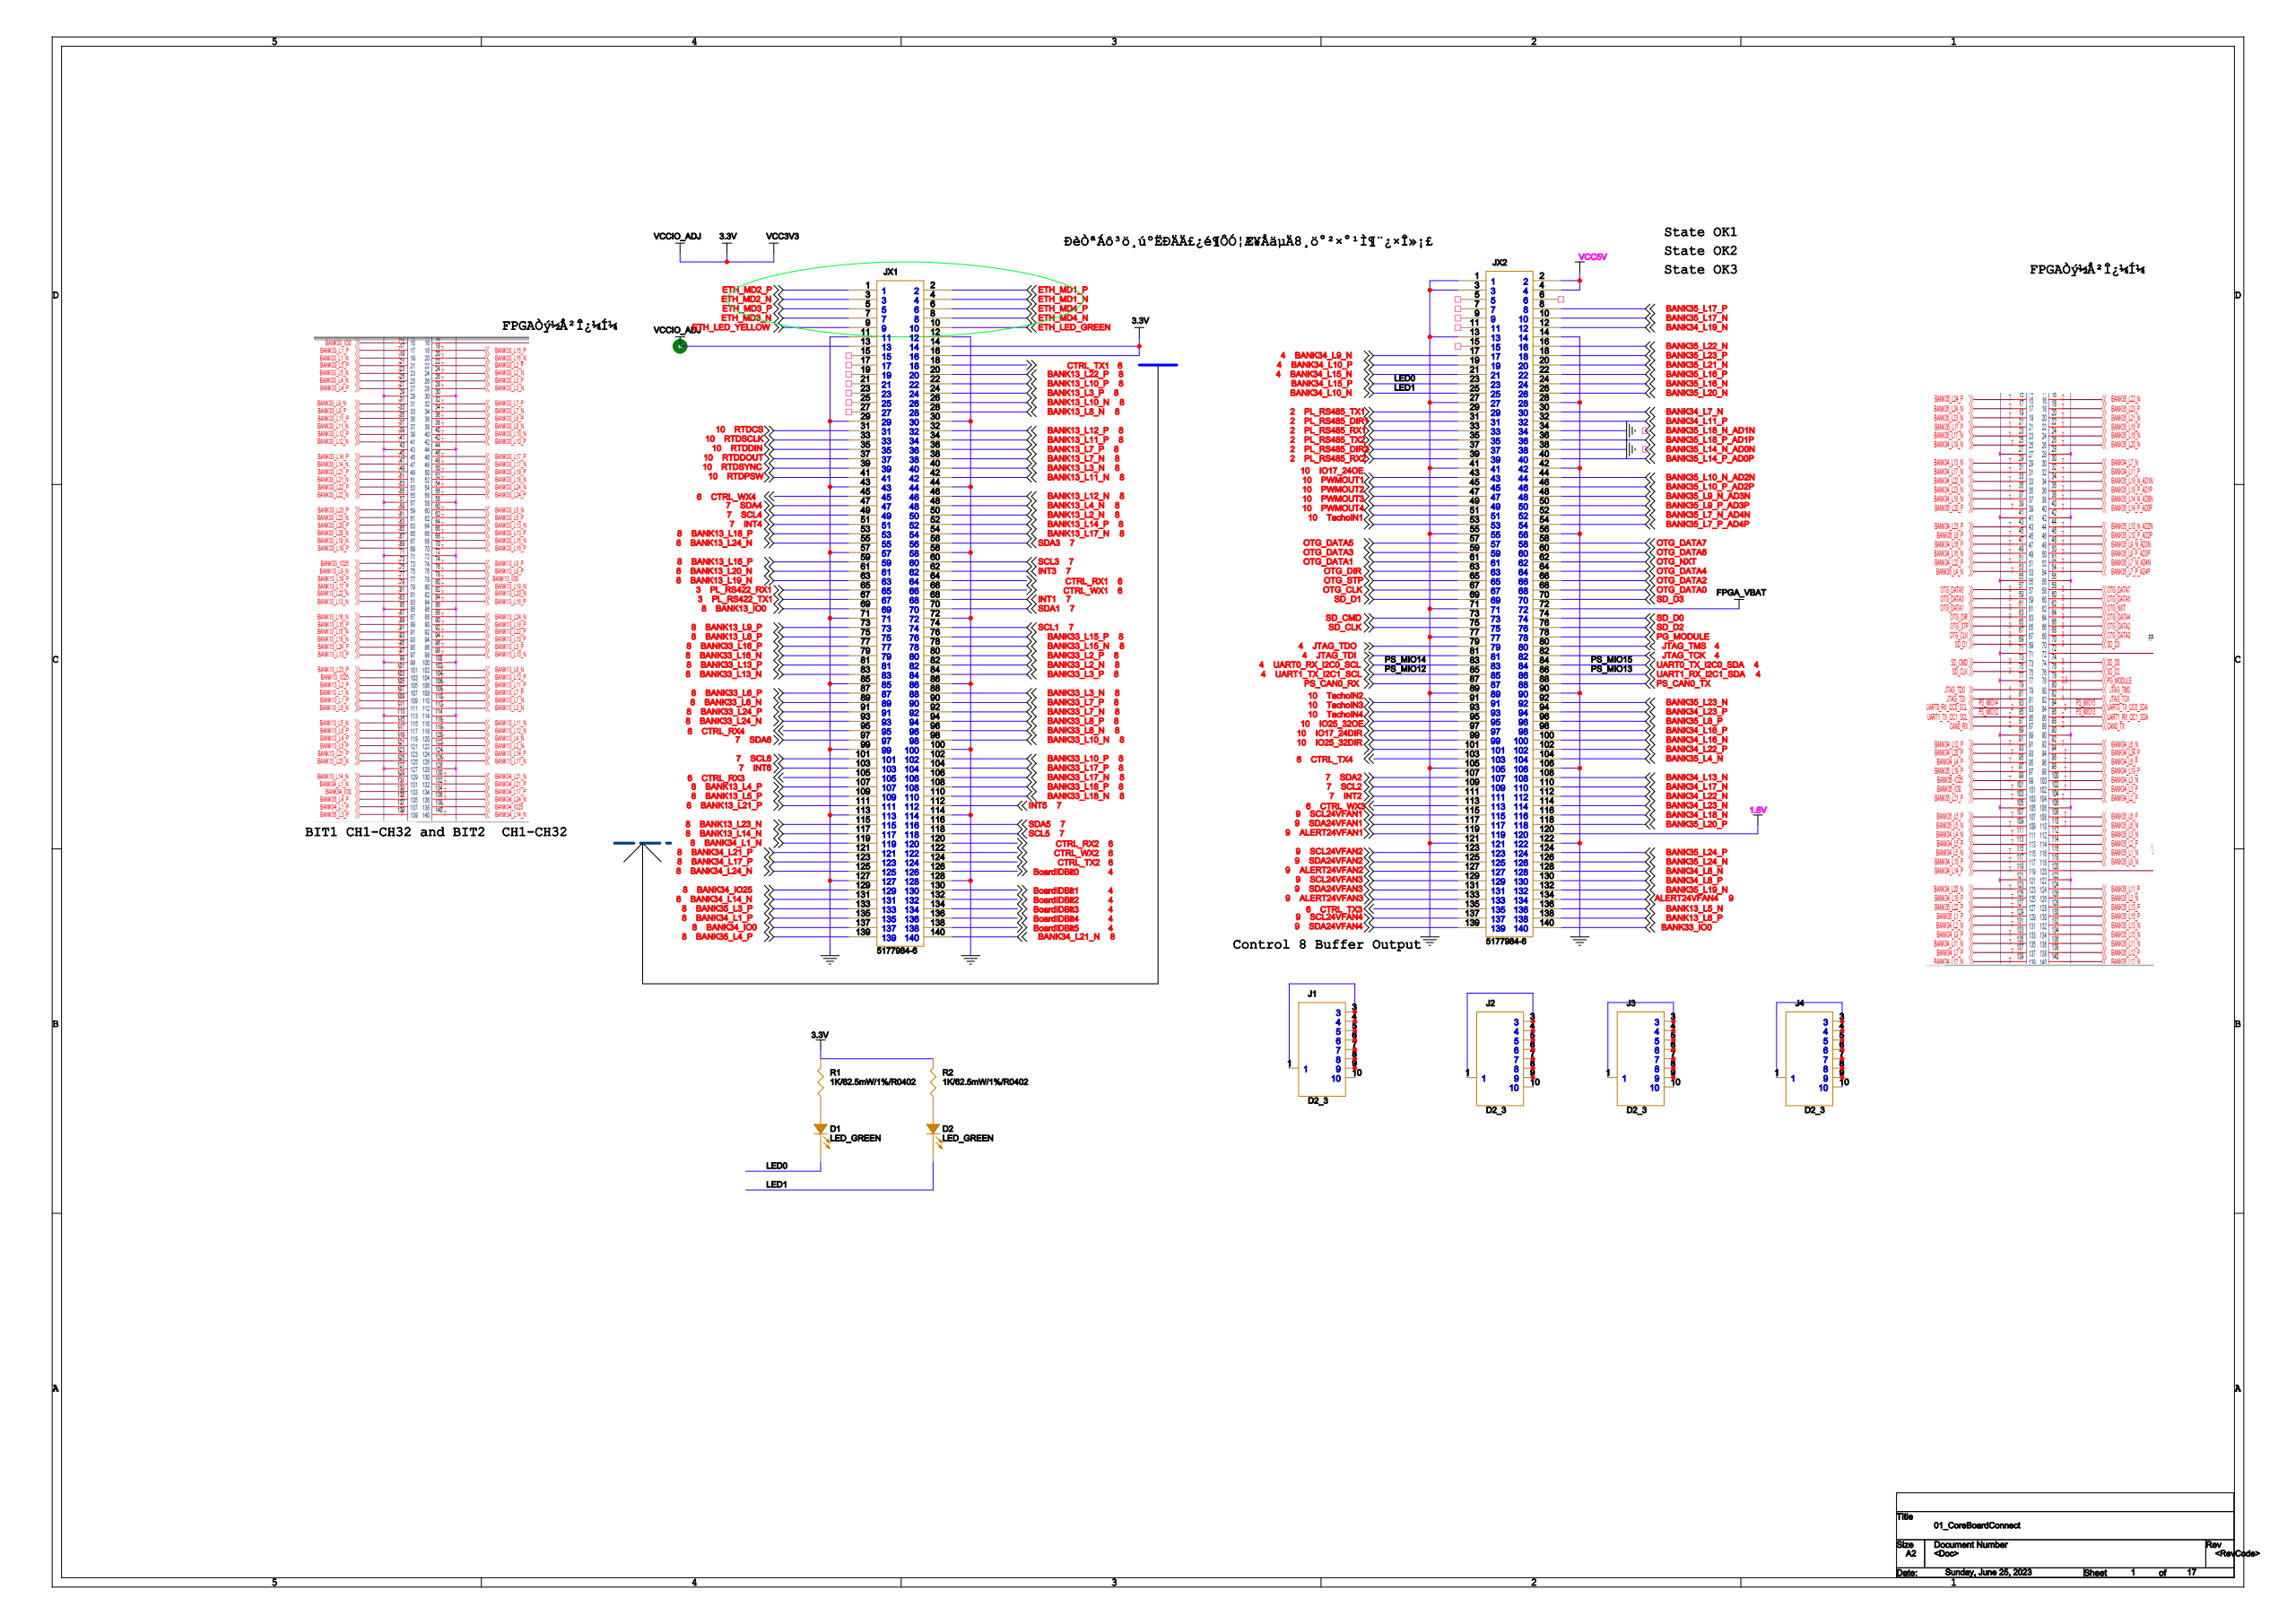Circuit board | Cadence Allegro | 2002 parts | 1538 nets | one sheet of the schematic
Parts on this sheet (reference | value | footprint):
D1 | LED_GREEN | LED0805
D2 | LED_GREEN | LED0805
J1 | D2_3 | D2_3
J2 | D2_3 | D2_3
J3 | D2_3 | D2_3
J4 | D2_3 | D2_3
JX1 | 5177984-6 | 5177983-6
JX2 | 5177984-6 | 5177983-6
R1 | 1K/62.5mW/1%/R0402 | 0402
R2 | 1K/62.5mW/1%/R0402 | 0402
Nets of these parts (net: part-pin ...):
3.3V: R1-2 R2-2 JX1-13 JX1-14 JX1-16
ETH_MD2_P: JX1-1
ETH_LED_GREEN: JX1-10
SCL6: JX1-101
BANK33_L10_P: JX1-102
INT6: JX1-103
BANK33_L17_P: JX1-104
CTRL_RX3: JX1-105
BANK33_L17_N: JX1-106
BANK13_L4_P: JX1-107
BANK33_L18_P: JX1-108
BANK13_L5_P: JX1-109
BANK33_L18_N: JX1-110
BANK13_L21_P: JX1-111
INT5: JX1-112
BANK13_L23_N: JX1-115
SDA5: JX1-116
BANK13_L14_N: JX1-117
SCL5: JX1-118
BANK34_L1_N: JX1-119
CTRL_RX2: JX1-120
BANK34_L21_P: JX1-121
CTRL_WX2: JX1-122
BANK34_L17_P: JX1-123
CTRL_TX2: JX1-124
BANK34_L24_N: JX1-125
BANK34_IO25: JX1-129
BANK34_L14_N: JX1-131
BANK35_L3_P: JX1-133
BANK34_L1_P: JX1-135
BANK34_IO0: JX1-137
BANK35_L4_P: JX1-139
BANK34_L21_N: JX1-140
CTRL_TX1: JX1-18
ETH_MD1_P: JX1-2
BANK13_L22_P: JX1-20
BANK13_L10_P: JX1-22
BANK13_L3_P: JX1-24
BANK13_L10_N: JX1-26
BANK13_L8_N: JX1-28
ETH_MD2_N: JX1-3
RTDCS: JX1-31
BANK13_L12_P: JX1-32
RTDSCLK: JX1-33
BANK13_L11_P: JX1-34
RTDDIN: JX1-35
BANK13_L7_P: JX1-36
RTDDOUT: JX1-37
BANK13_L7_N: JX1-38
RTDSYNC: JX1-39
ETH_MD1_N: JX1-4
BANK13_L3_N: JX1-40
RTDPSW: JX1-41
BANK13_L11_N: JX1-42
CTRL_WX4: JX1-45
BANK13_L12_N: JX1-46
SDA4: JX1-47
BANK13_L4_N: JX1-48
SCL4: JX1-49
ETH_MD3_P: JX1-5
BANK13_L2_N: JX1-50
INT4: JX1-51
BANK13_L14_P: JX1-52
BANK13_L18_P: JX1-53
BANK13_L17_N: JX1-54
BANK13_L24_N: JX1-55
SDA3: JX1-56
BANK13_L16_P: JX1-59
ETH_MD4_P: JX1-6
SCL3: JX1-60
BANK13_L20_N: JX1-61
INT3: JX1-62
BANK13_L19_N: JX1-63
CTRL_RX1: JX1-64
PL_RS422_RX1: JX1-65
CTRL_WX1: JX1-66
PL_RS422_TX1: JX1-67
INT1: JX1-68
BANK13_IO0: JX1-69
ETH_MD3_N: JX1-7
SDA1: JX1-70
BANK13_L9_P: JX1-73
SCL1: JX1-74
BANK13_L8_P: JX1-75
BANK33_L15_P: JX1-76
BANK33_L16_P: JX1-77
BANK33_L15_N: JX1-78
BANK33_L16_N: JX1-79
ETH_MD4_N: JX1-8
BANK33_L2_P: JX1-80
BANK33_L13_P: JX1-81
BANK33_L2_N: JX1-82
BANK33_L13_N: JX1-83
BANK33_L3_P: JX1-84
BANK33_L6_P: JX1-87
BANK33_L3_N: JX1-88
BANK33_L6_N: JX1-89
ETH_LED_YELLOW: JX1-9
BANK33_L7_P: JX1-90
BANK33_L24_P: JX1-91
BANK33_L7_N: JX1-92
BANK33_L24_N: JX1-93
BANK33_L8_P: JX1-94
CTRL_RX4: JX1-95
BANK33_L8_N: JX1-96
SDA6: JX1-97
BANK33_L10_N: JX1-98
BANK35_L17_N: JX2-10
BANK34_L16_N: JX2-100
IO25_32DIR: JX2-101
BANK34_L22_P: JX2-102
CTRL_TX4: JX2-103
BANK35_L4_N: JX2-104
SDA2: JX2-107
BANK34_L13_N: JX2-108
SCL2: JX2-109
BANK34_L17_N: JX2-110
INT2: JX2-111
BANK34_L22_N: JX2-112
CTRL_WX3: JX2-113
BANK34_L23_N: JX2-114
SCL24VFAN1: JX2-115
BANK34_L18_N: JX2-116
SDA24VFAN1: JX2-117
BANK35_L20_P: JX2-118
ALERT24VFAN1: JX2-119
BANK34_L19_N: JX2-12
1.8V: JX2-120
SCL24VFAN2: JX2-123
BANK35_L24_P: JX2-124
SDA24VFAN2: JX2-125
BANK35_L24_N: JX2-126
ALERT24VFAN2: JX2-127
BANK34_L8_N: JX2-128
SCL24VFAN3: JX2-129
BANK34_L8_P: JX2-130
SDA24VFAN3: JX2-131
BANK35_L19_N: JX2-132
ALERT24VFAN3: JX2-133
ALERT24VFAN4: JX2-134
CTRL_TX3: JX2-135
BANK13_L5_N: JX2-136
SCL24VFAN4: JX2-137
BANK13_L6_P: JX2-138
SDA24VFAN4: JX2-139
BANK33_IO0: JX2-140
BANK35_L22_N: JX2-16
BANK34_L9_N: JX2-17
BANK35_L23_P: JX2-18
BANK34_L10_P: JX2-19
VCC5V: JX2-2 JX2-4
BANK35_L21_N: JX2-20
BANK34_L15_N: JX2-21
BANK35_L16_P: JX2-22
BANK34_L15_P: D1-2 JX2-23
BANK35_L16_N: JX2-24
BANK34_L10_N: D2-2 JX2-25
BANK35_L20_N: JX2-26
PL_RS485_TX1: JX2-29
BANK34_L7_N: JX2-30
PL_RS485_DIR1: JX2-31
BANK34_L11_P: JX2-32
PL_RS485_RX1: JX2-33
PL_RS485_TX2: JX2-35
BANK35_L18_P_AD1P: JX2-36
PL_RS485_DIR2: JX2-37
PL_RS485_RX2: JX2-39
BANK35_L14_P_AD0P: JX2-40
IO17_24OE: JX2-43
BANK35_L10_N_AD2N: JX2-44
PWMOUT1: JX2-45
BANK35_L10_P_AD2P: JX2-46
PWMOUT2: JX2-47
BANK35_L9_N_AD3N: JX2-48
PWMOUT3: JX2-49
BANK35_L9_P_AD3P: JX2-50
PWMOUT4: JX2-51
BANK35_L7_N_AD4N: JX2-52
BANK35_L7_P_AD4P: JX2-54
OTG_DATA5: JX2-57
OTG_DATA7: JX2-58
OTG_DATA3: JX2-59
OTG_DATA6: JX2-60
OTG_DATA1: JX2-61
OTG_NXT: JX2-62
OTG_DIR: JX2-63
OTG_DATA4: JX2-64
OTG_STP: JX2-65
OTG_DATA2: JX2-66
OTG_CLK: JX2-67
OTG_DATA0: JX2-68
SD_D1: JX2-69
SD_D3: JX2-70
FPGA_VBAT: JX2-72
SD_CMD: JX2-73
SD_D0: JX2-74
SD_CLK: JX2-75
SD_D2: JX2-76
PG_MODULE: JX2-78
JTAG_TDO: JX2-79
BANK35_L17_P: JX2-8
JTAG_TMS: JX2-80
JTAG_TDI: JX2-81
JTAG_TCK: JX2-82
UART0_RX_I2C0_SCL: JX2-83
UART0_TX_I2C0_SDA: JX2-84
UART1_TX_I2C1_SCL: JX2-85
UART1_RX_I2C1_SDA: JX2-86
PS_CAN0_RX: JX2-87
PS_CAN0_TX: JX2-88
BANK35_L23_N: JX2-92
BANK34_L23_P: JX2-94
BANK35_L8_P: JX2-96
IO25_32OE: JX2-97
BANK34_L16_P: JX2-98
IO17_24DIR: JX2-99
N231084320: D1-1 R1-1
N231087860: D2-1 R2-1
N23884939: J1-1 J1-3 J1-4 J1-5 J1-6 J1-7 J1-8 J1-9 J1-10
N23884945: J2-1 J2-3 J2-4 J2-5 J2-6 J2-7 J2-8 J2-9 J2-10
N23884981: J3-1 J3-3 J3-4 J3-5 J3-6 J3-7 J3-8 J3-9 J3-10
N23884987: J4-1 J4-3 J4-4 J4-5 J4-6 J4-7 J4-8 J4-9 J4-10